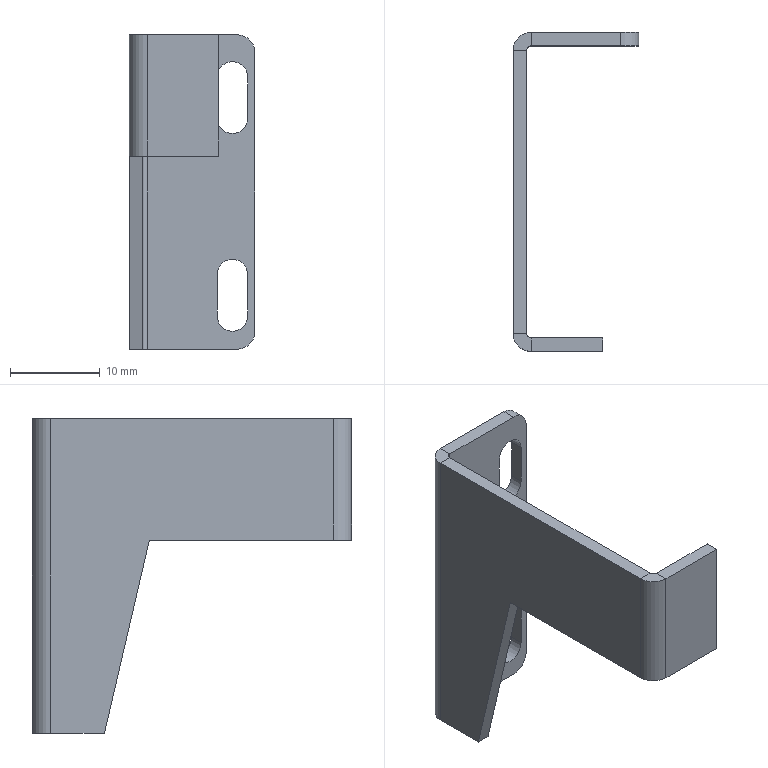Part | NX | features BREP 1 | 1 solid | 36 faces | box 14 x 35.5 x 35 mm | volume 1770 mm3 | plane 24 | cylinder 12 | commonest cylinder face diameters 3.4 x6 4 x4 1 x2
STEP:
#1=CARTESIAN_POINT('',(12.,0.,17.5));
#2=VERTEX_POINT('',#1);
#3=CARTESIAN_POINT('',(14.,0.,15.5));
#4=VERTEX_POINT('',#3);
#5=CARTESIAN_POINT('',(12.,0.,15.5));
#6=DIRECTION('',(0.,1.,0.));
#7=DIRECTION('',(0.,0.,1.));
#8=AXIS2_PLACEMENT_3D('',#5,#6,#7);
#9=CIRCLE('',#8,2.);
#10=EDGE_CURVE('',#2,#4,#9,.T.);
#11=ORIENTED_EDGE('',*,*,#10,.F.);
#12=CARTESIAN_POINT('',(12.,-1.5,17.5));
#13=VERTEX_POINT('',#12);
#14=CARTESIAN_POINT('',(12.,-2.,17.5));
#15=DIRECTION('',(0.,1.,0.));
#16=VECTOR('',#15,1000.);
#17=LINE('',#14,#16);
#18=EDGE_CURVE('',#13,#2,#17,.T.);
#19=ORIENTED_EDGE('',*,*,#18,.F.);
#20=CARTESIAN_POINT('',(14.,-1.5,15.5));
#21=VERTEX_POINT('',#20);
#22=CARTESIAN_POINT('',(12.,-1.5,15.5));
#23=DIRECTION('',(0.,-1.,0.));
#24=DIRECTION('',(0.,0.,1.));
#25=AXIS2_PLACEMENT_3D('',#22,#23,#24);
#26=CIRCLE('',#25,2.);
#27=EDGE_CURVE('',#21,#13,#26,.T.);
#28=ORIENTED_EDGE('',*,*,#27,.F.);
#29=CARTESIAN_POINT('',(14.,0.,15.5));
#30=DIRECTION('',(0.,-1.,0.));
#31=VECTOR('',#30,1000.);
#32=LINE('',#29,#31);
#33=EDGE_CURVE('',#4,#21,#32,.T.);
#34=ORIENTED_EDGE('',*,*,#33,.F.);
#35=EDGE_LOOP('',(#11,#19,#28,#34));
#36=FACE_BOUND('',#35,.T.);
#37=CARTESIAN_POINT('',(12.,0.,15.5));
#38=DIRECTION('',(0.,-1.,0.));
#39=DIRECTION('',(0.,0.,-1.));
#40=AXIS2_PLACEMENT_3D('',#37,#38,#39);
#41=CYLINDRICAL_SURFACE('',#40,2.);
#42=ADVANCED_FACE('',(#36),#41,.T.);
#43=CARTESIAN_POINT('',(14.,0.,-15.5));
#44=VERTEX_POINT('',#43);
#45=CARTESIAN_POINT('',(12.,0.,-17.5));
#46=VERTEX_POINT('',#45);
#47=CARTESIAN_POINT('',(12.,0.,-15.5));
#48=DIRECTION('',(0.,1.,0.));
#49=DIRECTION('',(0.,0.,1.));
#50=AXIS2_PLACEMENT_3D('',#47,#48,#49);
#51=CIRCLE('',#50,2.);
#52=EDGE_CURVE('',#44,#46,#51,.T.);
#53=ORIENTED_EDGE('',*,*,#52,.F.);
#54=CARTESIAN_POINT('',(14.,-1.5,-15.5));
#55=VERTEX_POINT('',#54);
#56=CARTESIAN_POINT('',(14.,0.,-15.5));
#57=DIRECTION('',(0.,1.,0.));
#58=VECTOR('',#57,1000.);
#59=LINE('',#56,#58);
#60=EDGE_CURVE('',#55,#44,#59,.T.);
#61=ORIENTED_EDGE('',*,*,#60,.F.);
#62=CARTESIAN_POINT('',(12.,-1.5,-17.5));
#63=VERTEX_POINT('',#62);
#64=CARTESIAN_POINT('',(12.,-1.5,-15.5));
#65=DIRECTION('',(0.,-1.,0.));
#66=DIRECTION('',(0.,0.,1.));
#67=AXIS2_PLACEMENT_3D('',#64,#65,#66);
#68=CIRCLE('',#67,2.);
#69=EDGE_CURVE('',#63,#55,#68,.T.);
#70=ORIENTED_EDGE('',*,*,#69,.F.);
#71=CARTESIAN_POINT('',(12.,-1.5,-17.5));
#72=DIRECTION('',(0.,-1.,0.));
#73=VECTOR('',#72,1000.);
#74=LINE('',#71,#73);
#75=EDGE_CURVE('',#46,#63,#74,.T.);
#76=ORIENTED_EDGE('',*,*,#75,.F.);
#77=EDGE_LOOP('',(#53,#61,#70,#76));
#78=FACE_BOUND('',#77,.T.);
#79=CARTESIAN_POINT('',(12.,-2.,-15.5));
#80=DIRECTION('',(0.,1.,0.));
#81=DIRECTION('',(0.,0.,1.));
#82=AXIS2_PLACEMENT_3D('',#79,#80,#81);
#83=CYLINDRICAL_SURFACE('',#82,2.);
#84=ADVANCED_FACE('',(#78),#83,.T.);
#85=CARTESIAN_POINT('',(13.2,0.,-9.2));
#86=VERTEX_POINT('',#85);
#87=CARTESIAN_POINT('',(13.2,-1.5,-9.2));
#88=VERTEX_POINT('',#87);
#89=CARTESIAN_POINT('',(13.2,-1.501,-9.2));
#90=DIRECTION('',(0.,-1.,0.));
#91=VECTOR('',#90,1000.);
#92=LINE('',#89,#91);
#93=EDGE_CURVE('',#86,#88,#92,.T.);
#94=ORIENTED_EDGE('',*,*,#93,.F.);
#95=CARTESIAN_POINT('',(13.2,0.,-13.8));
#96=VERTEX_POINT('',#95);
#97=CARTESIAN_POINT('',(13.2,0.,-9.2));
#98=DIRECTION('',(0.,0.,-1.));
#99=VECTOR('',#98,1000.);
#100=LINE('',#97,#99);
#101=EDGE_CURVE('',#86,#96,#100,.T.);
#102=ORIENTED_EDGE('',*,*,#101,.T.);
#103=CARTESIAN_POINT('',(13.2,-1.5,-13.8));
#104=VERTEX_POINT('',#103);
#105=CARTESIAN_POINT('',(13.2,-1.501,-13.8));
#106=DIRECTION('',(0.,-1.,0.));
#107=VECTOR('',#106,1000.);
#108=LINE('',#105,#107);
#109=EDGE_CURVE('',#96,#104,#108,.T.);
#110=ORIENTED_EDGE('',*,*,#109,.T.);
#111=CARTESIAN_POINT('',(13.2,-1.5,17.5));
#112=DIRECTION('',(0.,0.,-1.));
#113=VECTOR('',#112,1000.);
#114=LINE('',#111,#113);
#115=EDGE_CURVE('',#88,#104,#114,.T.);
#116=ORIENTED_EDGE('',*,*,#115,.F.);
#117=EDGE_LOOP('',(#94,#102,#110,#116));
#118=FACE_BOUND('',#117,.T.);
#119=CARTESIAN_POINT('',(13.2,-1.501,-9.2));
#120=DIRECTION('',(1.,0.,0.));
#121=DIRECTION('',(0.,1.,0.));
#122=AXIS2_PLACEMENT_3D('',#119,#120,#121);
#123=PLANE('',#122);
#124=ADVANCED_FACE('',(#118),#123,.F.);
#125=CARTESIAN_POINT('',(9.8,-1.5,-13.8));
#126=VERTEX_POINT('',#125);
#127=CARTESIAN_POINT('',(9.8,0.,-13.8));
#128=VERTEX_POINT('',#127);
#129=CARTESIAN_POINT('',(9.8,0.,-13.8));
#130=DIRECTION('',(0.,1.,0.));
#131=VECTOR('',#130,1000.);
#132=LINE('',#129,#131);
#133=EDGE_CURVE('',#126,#128,#132,.T.);
#134=ORIENTED_EDGE('',*,*,#133,.T.);
#135=CARTESIAN_POINT('',(9.8,0.,-9.2));
#136=VERTEX_POINT('',#135);
#137=CARTESIAN_POINT('',(9.8,0.,-9.2));
#138=DIRECTION('',(0.,0.,-1.));
#139=VECTOR('',#138,1000.);
#140=LINE('',#137,#139);
#141=EDGE_CURVE('',#136,#128,#140,.T.);
#142=ORIENTED_EDGE('',*,*,#141,.F.);
#143=CARTESIAN_POINT('',(9.8,-1.5,-9.2));
#144=VERTEX_POINT('',#143);
#145=CARTESIAN_POINT('',(9.8,0.,-9.2));
#146=DIRECTION('',(0.,-1.,0.));
#147=VECTOR('',#146,1000.);
#148=LINE('',#145,#147);
#149=EDGE_CURVE('',#136,#144,#148,.T.);
#150=ORIENTED_EDGE('',*,*,#149,.T.);
#151=CARTESIAN_POINT('',(9.8,-1.5,17.5));
#152=DIRECTION('',(0.,0.,1.));
#153=VECTOR('',#152,1000.);
#154=LINE('',#151,#153);
#155=EDGE_CURVE('',#126,#144,#154,.T.);
#156=ORIENTED_EDGE('',*,*,#155,.F.);
#157=EDGE_LOOP('',(#134,#142,#150,#156));
#158=FACE_BOUND('',#157,.T.);
#159=CARTESIAN_POINT('',(9.8,0.,-9.2));
#160=DIRECTION('',(-1.,0.,0.));
#161=DIRECTION('',(0.,0.,1.));
#162=AXIS2_PLACEMENT_3D('',#159,#160,#161);
#163=PLANE('',#162);
#164=ADVANCED_FACE('',(#158),#163,.F.);
#165=CARTESIAN_POINT('',(11.5,-1.5,-7.5));
#166=VERTEX_POINT('',#165);
#167=CARTESIAN_POINT('',(11.5,0.,-7.5));
#168=VERTEX_POINT('',#167);
#169=CARTESIAN_POINT('',(11.5,0.,-7.5));
#170=DIRECTION('',(0.,1.,0.));
#171=VECTOR('',#170,1000.);
#172=LINE('',#169,#171);
#173=EDGE_CURVE('',#166,#168,#172,.T.);
#174=ORIENTED_EDGE('',*,*,#173,.F.);
#175=CARTESIAN_POINT('',(11.5,-1.5,-9.2));
#176=DIRECTION('',(0.,1.,0.));
#177=DIRECTION('',(0.,0.,1.));
#178=AXIS2_PLACEMENT_3D('',#175,#176,#177);
#179=CIRCLE('',#178,1.7);
#180=EDGE_CURVE('',#144,#166,#179,.T.);
#181=ORIENTED_EDGE('',*,*,#180,.F.);
#182=ORIENTED_EDGE('',*,*,#149,.F.);
#183=CARTESIAN_POINT('',(11.5,0.,-9.2));
#184=DIRECTION('',(0.,1.,0.));
#185=DIRECTION('',(0.,0.,1.));
#186=AXIS2_PLACEMENT_3D('',#183,#184,#185);
#187=CIRCLE('',#186,1.7);
#188=EDGE_CURVE('',#136,#168,#187,.T.);
#189=ORIENTED_EDGE('',*,*,#188,.T.);
#190=EDGE_LOOP('',(#174,#181,#182,#189));
#191=FACE_BOUND('',#190,.T.);
#192=CARTESIAN_POINT('',(11.5,0.,-9.2));
#193=DIRECTION('',(0.,1.,0.));
#194=DIRECTION('',(0.,0.,1.));
#195=AXIS2_PLACEMENT_3D('',#192,#193,#194);
#196=CYLINDRICAL_SURFACE('',#195,1.7);
#197=ADVANCED_FACE('',(#191),#196,.F.);
#198=ORIENTED_EDGE('',*,*,#109,.F.);
#199=CARTESIAN_POINT('',(11.5,0.,-13.8));
#200=DIRECTION('',(0.,1.,0.));
#201=DIRECTION('',(0.,0.,1.));
#202=AXIS2_PLACEMENT_3D('',#199,#200,#201);
#203=CIRCLE('',#202,1.7);
#204=EDGE_CURVE('',#96,#128,#203,.T.);
#205=ORIENTED_EDGE('',*,*,#204,.T.);
#206=ORIENTED_EDGE('',*,*,#133,.F.);
#207=CARTESIAN_POINT('',(11.5,-1.5,-13.8));
#208=DIRECTION('',(0.,1.,0.));
#209=DIRECTION('',(0.,0.,1.));
#210=AXIS2_PLACEMENT_3D('',#207,#208,#209);
#211=CIRCLE('',#210,1.7);
#212=EDGE_CURVE('',#104,#126,#211,.T.);
#213=ORIENTED_EDGE('',*,*,#212,.F.);
#214=EDGE_LOOP('',(#198,#205,#206,#213));
#215=FACE_BOUND('',#214,.T.);
#216=CARTESIAN_POINT('',(11.5,0.,-13.8));
#217=DIRECTION('',(0.,1.,0.));
#218=DIRECTION('',(0.,0.,1.));
#219=AXIS2_PLACEMENT_3D('',#216,#217,#218);
#220=CYLINDRICAL_SURFACE('',#219,1.7);
#221=ADVANCED_FACE('',(#215),#220,.F.);
#222=CARTESIAN_POINT('',(13.2,0.,12.8));
#223=VERTEX_POINT('',#222);
#224=CARTESIAN_POINT('',(13.2,-1.5,12.8));
#225=VERTEX_POINT('',#224);
#226=CARTESIAN_POINT('',(13.2,-1.501,12.8));
#227=DIRECTION('',(0.,-1.,0.));
#228=VECTOR('',#227,1000.);
#229=LINE('',#226,#228);
#230=EDGE_CURVE('',#223,#225,#229,.T.);
#231=ORIENTED_EDGE('',*,*,#230,.F.);
#232=CARTESIAN_POINT('',(13.2,0.,8.2));
#233=VERTEX_POINT('',#232);
#234=CARTESIAN_POINT('',(13.2,0.,12.8));
#235=DIRECTION('',(0.,0.,-1.));
#236=VECTOR('',#235,1000.);
#237=LINE('',#234,#236);
#238=EDGE_CURVE('',#223,#233,#237,.T.);
#239=ORIENTED_EDGE('',*,*,#238,.T.);
#240=CARTESIAN_POINT('',(13.2,-1.5,8.2));
#241=VERTEX_POINT('',#240);
#242=CARTESIAN_POINT('',(13.2,-1.501,8.2));
#243=DIRECTION('',(0.,-1.,0.));
#244=VECTOR('',#243,1000.);
#245=LINE('',#242,#244);
#246=EDGE_CURVE('',#233,#241,#245,.T.);
#247=ORIENTED_EDGE('',*,*,#246,.T.);
#248=CARTESIAN_POINT('',(13.2,-1.5,17.5));
#249=DIRECTION('',(0.,0.,-1.));
#250=VECTOR('',#249,1000.);
#251=LINE('',#248,#250);
#252=EDGE_CURVE('',#225,#241,#251,.T.);
#253=ORIENTED_EDGE('',*,*,#252,.F.);
#254=EDGE_LOOP('',(#231,#239,#247,#253));
#255=FACE_BOUND('',#254,.T.);
#256=CARTESIAN_POINT('',(13.2,-1.501,12.8));
#257=DIRECTION('',(1.,0.,0.));
#258=DIRECTION('',(0.,1.,0.));
#259=AXIS2_PLACEMENT_3D('',#256,#257,#258);
#260=PLANE('',#259);
#261=ADVANCED_FACE('',(#255),#260,.F.);
#262=CARTESIAN_POINT('',(9.8,-1.5,8.2));
#263=VERTEX_POINT('',#262);
#264=CARTESIAN_POINT('',(9.8,0.,8.2));
#265=VERTEX_POINT('',#264);
#266=CARTESIAN_POINT('',(9.8,0.,8.2));
#267=DIRECTION('',(0.,1.,0.));
#268=VECTOR('',#267,1000.);
#269=LINE('',#266,#268);
#270=EDGE_CURVE('',#263,#265,#269,.T.);
#271=ORIENTED_EDGE('',*,*,#270,.T.);
#272=CARTESIAN_POINT('',(9.8,0.,12.8));
#273=VERTEX_POINT('',#272);
#274=CARTESIAN_POINT('',(9.8,0.,12.8));
#275=DIRECTION('',(0.,0.,-1.));
#276=VECTOR('',#275,1000.);
#277=LINE('',#274,#276);
#278=EDGE_CURVE('',#273,#265,#277,.T.);
#279=ORIENTED_EDGE('',*,*,#278,.F.);
#280=CARTESIAN_POINT('',(9.8,-1.5,12.8));
#281=VERTEX_POINT('',#280);
#282=CARTESIAN_POINT('',(9.8,0.,12.8));
#283=DIRECTION('',(0.,-1.,0.));
#284=VECTOR('',#283,1000.);
#285=LINE('',#282,#284);
#286=EDGE_CURVE('',#273,#281,#285,.T.);
#287=ORIENTED_EDGE('',*,*,#286,.T.);
#288=CARTESIAN_POINT('',(9.8,-1.5,17.5));
#289=DIRECTION('',(0.,0.,1.));
#290=VECTOR('',#289,1000.);
#291=LINE('',#288,#290);
#292=EDGE_CURVE('',#263,#281,#291,.T.);
#293=ORIENTED_EDGE('',*,*,#292,.F.);
#294=EDGE_LOOP('',(#271,#279,#287,#293));
#295=FACE_BOUND('',#294,.T.);
#296=CARTESIAN_POINT('',(9.8,0.,12.8));
#297=DIRECTION('',(-1.,0.,0.));
#298=DIRECTION('',(0.,0.,1.));
#299=AXIS2_PLACEMENT_3D('',#296,#297,#298);
#300=PLANE('',#299);
#301=ADVANCED_FACE('',(#295),#300,.F.);
#302=CARTESIAN_POINT('',(11.5,-1.5,14.5));
#303=VERTEX_POINT('',#302);
#304=CARTESIAN_POINT('',(11.5,0.,14.5));
#305=VERTEX_POINT('',#304);
#306=CARTESIAN_POINT('',(11.5,0.,14.5));
#307=DIRECTION('',(0.,1.,0.));
#308=VECTOR('',#307,1000.);
#309=LINE('',#306,#308);
#310=EDGE_CURVE('',#303,#305,#309,.T.);
#311=ORIENTED_EDGE('',*,*,#310,.F.);
#312=CARTESIAN_POINT('',(11.5,-1.5,12.8));
#313=DIRECTION('',(0.,1.,0.));
#314=DIRECTION('',(0.,0.,1.));
#315=AXIS2_PLACEMENT_3D('',#312,#313,#314);
#316=CIRCLE('',#315,1.7);
#317=EDGE_CURVE('',#281,#303,#316,.T.);
#318=ORIENTED_EDGE('',*,*,#317,.F.);
#319=ORIENTED_EDGE('',*,*,#286,.F.);
#320=CARTESIAN_POINT('',(11.5,0.,12.8));
#321=DIRECTION('',(0.,1.,0.));
#322=DIRECTION('',(0.,0.,1.));
#323=AXIS2_PLACEMENT_3D('',#320,#321,#322);
#324=CIRCLE('',#323,1.7);
#325=EDGE_CURVE('',#273,#305,#324,.T.);
#326=ORIENTED_EDGE('',*,*,#325,.T.);
#327=EDGE_LOOP('',(#311,#318,#319,#326));
#328=FACE_BOUND('',#327,.T.);
#329=CARTESIAN_POINT('',(11.5,0.,12.8));
#330=DIRECTION('',(0.,1.,0.));
#331=DIRECTION('',(0.,0.,1.));
#332=AXIS2_PLACEMENT_3D('',#329,#330,#331);
#333=CYLINDRICAL_SURFACE('',#332,1.7);
#334=ADVANCED_FACE('',(#328),#333,.F.);
#335=ORIENTED_EDGE('',*,*,#246,.F.);
#336=CARTESIAN_POINT('',(11.5,0.,8.2));
#337=DIRECTION('',(0.,1.,0.));
#338=DIRECTION('',(0.,0.,1.));
#339=AXIS2_PLACEMENT_3D('',#336,#337,#338);
#340=CIRCLE('',#339,1.7);
#341=EDGE_CURVE('',#233,#265,#340,.T.);
#342=ORIENTED_EDGE('',*,*,#341,.T.);
#343=ORIENTED_EDGE('',*,*,#270,.F.);
#344=CARTESIAN_POINT('',(11.5,-1.5,8.2));
#345=DIRECTION('',(0.,1.,0.));
#346=DIRECTION('',(0.,0.,1.));
#347=AXIS2_PLACEMENT_3D('',#344,#345,#346);
#348=CIRCLE('',#347,1.7);
#349=EDGE_CURVE('',#241,#263,#348,.T.);
#350=ORIENTED_EDGE('',*,*,#349,.F.);
#351=EDGE_LOOP('',(#335,#342,#343,#350));
#352=FACE_BOUND('',#351,.T.);
#353=CARTESIAN_POINT('',(11.5,0.,8.2));
#354=DIRECTION('',(0.,1.,0.));
#355=DIRECTION('',(0.,0.,1.));
#356=AXIS2_PLACEMENT_3D('',#353,#354,#355);
#357=CYLINDRICAL_SURFACE('',#356,1.7);
#358=ADVANCED_FACE('',(#352),#357,.F.);
#359=CARTESIAN_POINT('',(2.,-35.5,4.));
#360=VERTEX_POINT('',#359);
#361=CARTESIAN_POINT('',(2.,-34.,4.));
#362=VERTEX_POINT('',#361);
#363=CARTESIAN_POINT('',(2.,-35.5,4.));
#364=DIRECTION('',(0.,1.,0.));
#365=VECTOR('',#364,1000.);
#366=LINE('',#363,#365);
#367=EDGE_CURVE('',#360,#362,#366,.T.);
#368=ORIENTED_EDGE('',*,*,#367,.F.);
#369=CARTESIAN_POINT('',(0.,-33.5,4.));
#370=VERTEX_POINT('',#369);
#371=CARTESIAN_POINT('',(2.,-33.5,4.));
#372=DIRECTION('',(0.,0.,1.));
#373=DIRECTION('',(0.,1.,0.));
#374=AXIS2_PLACEMENT_3D('',#371,#372,#373);
#375=CIRCLE('',#374,2.);
#376=EDGE_CURVE('',#370,#360,#375,.T.);
#377=ORIENTED_EDGE('',*,*,#376,.F.);
#378=CARTESIAN_POINT('',(1.5,-33.5,4.));
#379=VERTEX_POINT('',#378);
#380=CARTESIAN_POINT('',(1.5,-33.5,4.));
#381=DIRECTION('',(-1.,0.,0.));
#382=VECTOR('',#381,1000.);
#383=LINE('',#380,#382);
#384=EDGE_CURVE('',#379,#370,#383,.T.);
#385=ORIENTED_EDGE('',*,*,#384,.F.);
#386=CARTESIAN_POINT('',(2.,-33.5,4.));
#387=DIRECTION('',(0.,0.,1.));
#388=DIRECTION('',(-1.,0.,0.));
#389=AXIS2_PLACEMENT_3D('',#386,#387,#388);
#390=CIRCLE('',#389,0.5);
#391=EDGE_CURVE('',#379,#362,#390,.T.);
#392=ORIENTED_EDGE('',*,*,#391,.T.);
#393=EDGE_LOOP('',(#368,#377,#385,#392));
#394=FACE_BOUND('',#393,.T.);
#395=CARTESIAN_POINT('',(2.,-33.5,4.));
#396=DIRECTION('',(0.,0.,1.));
#397=DIRECTION('',(0.,-1.,0.));
#398=AXIS2_PLACEMENT_3D('',#395,#396,#397);
#399=PLANE('',#398);
#400=ADVANCED_FACE('',(#394),#399,.F.);
#401=CARTESIAN_POINT('',(10.,-35.5,4.));
#402=VERTEX_POINT('',#401);
#403=CARTESIAN_POINT('',(10.,-34.,4.));
#404=VERTEX_POINT('',#403);
#405=CARTESIAN_POINT('',(10.,-35.5,4.));
#406=DIRECTION('',(0.,1.,0.));
#407=VECTOR('',#406,1000.);
#408=LINE('',#405,#407);
#409=EDGE_CURVE('',#402,#404,#408,.T.);
#410=ORIENTED_EDGE('',*,*,#409,.F.);
#411=CARTESIAN_POINT('',(14.,-35.5,4.));
#412=DIRECTION('',(-1.,0.,0.));
#413=VECTOR('',#412,1000.);
#414=LINE('',#411,#413);
#415=EDGE_CURVE('',#402,#360,#414,.T.);
#416=ORIENTED_EDGE('',*,*,#415,.T.);
#417=ORIENTED_EDGE('',*,*,#367,.T.);
#418=CARTESIAN_POINT('',(0.,-34.,4.));
#419=DIRECTION('',(-1.,0.,0.));
#420=VECTOR('',#419,1000.);
#421=LINE('',#418,#420);
#422=EDGE_CURVE('',#404,#362,#421,.T.);
#423=ORIENTED_EDGE('',*,*,#422,.F.);
#424=EDGE_LOOP('',(#410,#416,#417,#423));
#425=FACE_BOUND('',#424,.T.);
#426=CARTESIAN_POINT('',(14.,-35.5,4.));
#427=DIRECTION('',(0.,0.,1.));
#428=DIRECTION('',(-1.,0.,0.));
#429=AXIS2_PLACEMENT_3D('',#426,#427,#428);
#430=PLANE('',#429);
#431=ADVANCED_FACE('',(#425),#430,.F.);
#432=CARTESIAN_POINT('',(1.5,-8.,-17.5));
#433=VERTEX_POINT('',#432);
#434=CARTESIAN_POINT('',(1.5,-13.,4.));
#435=VERTEX_POINT('',#434);
#436=CARTESIAN_POINT('',(1.5,-15.311,13.939));
#437=DIRECTION('',(0.,-0.2265,0.974));
#438=VECTOR('',#437,1000.);
#439=LINE('',#436,#438);
#440=EDGE_CURVE('',#433,#435,#439,.T.);
#441=ORIENTED_EDGE('',*,*,#440,.T.);
#442=CARTESIAN_POINT('',(0.,-13.,4.));
#443=VERTEX_POINT('',#442);
#444=CARTESIAN_POINT('',(1.5,-13.,4.));
#445=DIRECTION('',(-1.,0.,0.));
#446=VECTOR('',#445,1000.);
#447=LINE('',#444,#446);
#448=EDGE_CURVE('',#435,#443,#447,.T.);
#449=ORIENTED_EDGE('',*,*,#448,.T.);
#450=CARTESIAN_POINT('',(0.,-8.,-17.5));
#451=VERTEX_POINT('',#450);
#452=CARTESIAN_POINT('',(0.,-15.311,13.939));
#453=DIRECTION('',(0.,-0.2265,0.974));
#454=VECTOR('',#453,1000.);
#455=LINE('',#452,#454);
#456=EDGE_CURVE('',#451,#443,#455,.T.);
#457=ORIENTED_EDGE('',*,*,#456,.F.);
#458=CARTESIAN_POINT('',(1.5,-8.,-17.5));
#459=DIRECTION('',(-1.,0.,0.));
#460=VECTOR('',#459,1000.);
#461=LINE('',#458,#460);
#462=EDGE_CURVE('',#433,#451,#461,.T.);
#463=ORIENTED_EDGE('',*,*,#462,.F.);
#464=EDGE_LOOP('',(#441,#449,#457,#463));
#465=FACE_BOUND('',#464,.T.);
#466=CARTESIAN_POINT('',(1.5,-15.311,13.939));
#467=DIRECTION('',(0.,-0.974,-0.2265));
#468=DIRECTION('',(0.,-0.2265,0.974));
#469=AXIS2_PLACEMENT_3D('',#466,#467,#468);
#470=PLANE('',#469);
#471=ADVANCED_FACE('',(#465),#470,.T.);
#472=ORIENTED_EDGE('',*,*,#448,.F.);
#473=CARTESIAN_POINT('',(1.5,0.,4.));
#474=DIRECTION('',(0.,-1.,0.));
#475=VECTOR('',#474,1000.);
#476=LINE('',#473,#475);
#477=EDGE_CURVE('',#435,#379,#476,.T.);
#478=ORIENTED_EDGE('',*,*,#477,.T.);
#479=ORIENTED_EDGE('',*,*,#384,.T.);
#480=CARTESIAN_POINT('',(0.,0.,4.));
#481=DIRECTION('',(0.,-1.,0.));
#482=VECTOR('',#481,1000.);
#483=LINE('',#480,#482);
#484=EDGE_CURVE('',#443,#370,#483,.T.);
#485=ORIENTED_EDGE('',*,*,#484,.F.);
#486=EDGE_LOOP('',(#472,#478,#479,#485));
#487=FACE_BOUND('',#486,.T.);
#488=CARTESIAN_POINT('',(1.5,0.,4.));
#489=DIRECTION('',(0.,0.,-1.));
#490=DIRECTION('',(0.,-1.,0.));
#491=AXIS2_PLACEMENT_3D('',#488,#489,#490);
#492=PLANE('',#491);
#493=ADVANCED_FACE('',(#487),#492,.T.);
#494=CARTESIAN_POINT('',(2.,0.,-17.5));
#495=VERTEX_POINT('',#494);
#496=CARTESIAN_POINT('',(0.,0.,-17.5));
#497=DIRECTION('',(1.,0.,0.));
#498=VECTOR('',#497,1000.);
#499=LINE('',#496,#498);
#500=EDGE_CURVE('',#495,#46,#499,.T.);
#501=ORIENTED_EDGE('',*,*,#500,.T.);
#502=ORIENTED_EDGE('',*,*,#75,.T.);
#503=CARTESIAN_POINT('',(2.,-1.5,-17.5));
#504=VERTEX_POINT('',#503);
#505=CARTESIAN_POINT('',(0.,-1.5,-17.5));
#506=DIRECTION('',(1.,0.,0.));
#507=VECTOR('',#506,1000.);
#508=LINE('',#505,#507);
#509=EDGE_CURVE('',#504,#63,#508,.T.);
#510=ORIENTED_EDGE('',*,*,#509,.F.);
#511=CARTESIAN_POINT('',(2.,-1.5,-17.5));
#512=DIRECTION('',(0.,1.,0.));
#513=VECTOR('',#512,1000.);
#514=LINE('',#511,#513);
#515=EDGE_CURVE('',#504,#495,#514,.T.);
#516=ORIENTED_EDGE('',*,*,#515,.T.);
#517=EDGE_LOOP('',(#501,#502,#510,#516));
#518=FACE_BOUND('',#517,.T.);
#519=CARTESIAN_POINT('',(2.,-2.,-17.5));
#520=DIRECTION('',(0.,0.,1.));
#521=DIRECTION('',(1.,0.,0.));
#522=AXIS2_PLACEMENT_3D('',#519,#520,#521);
#523=PLANE('',#522);
#524=ADVANCED_FACE('',(#518),#523,.F.);
#525=CARTESIAN_POINT('',(10.,-34.,17.5));
#526=VERTEX_POINT('',#525);
#527=CARTESIAN_POINT('',(2.,-34.,17.5));
#528=VERTEX_POINT('',#527);
#529=CARTESIAN_POINT('',(0.,-34.,17.5));
#530=DIRECTION('',(-1.,0.,0.));
#531=VECTOR('',#530,1000.);
#532=LINE('',#529,#531);
#533=EDGE_CURVE('',#526,#528,#532,.T.);
#534=ORIENTED_EDGE('',*,*,#533,.T.);
#535=CARTESIAN_POINT('',(2.,-35.5,17.5));
#536=VERTEX_POINT('',#535);
#537=CARTESIAN_POINT('',(2.,-34.,17.5));
#538=DIRECTION('',(0.,-1.,0.));
#539=VECTOR('',#538,1000.);
#540=LINE('',#537,#539);
#541=EDGE_CURVE('',#528,#536,#540,.T.);
#542=ORIENTED_EDGE('',*,*,#541,.T.);
#543=CARTESIAN_POINT('',(10.,-35.5,17.5));
#544=VERTEX_POINT('',#543);
#545=CARTESIAN_POINT('',(0.,-35.5,17.5));
#546=DIRECTION('',(-1.,0.,0.));
#547=VECTOR('',#546,1000.);
#548=LINE('',#545,#547);
#549=EDGE_CURVE('',#544,#536,#548,.T.);
#550=ORIENTED_EDGE('',*,*,#549,.F.);
#551=CARTESIAN_POINT('',(10.,-34.,17.5));
#552=DIRECTION('',(0.,-1.,0.));
#553=VECTOR('',#552,1000.);
#554=LINE('',#551,#553);
#555=EDGE_CURVE('',#526,#544,#554,.T.);
#556=ORIENTED_EDGE('',*,*,#555,.F.);
#557=EDGE_LOOP('',(#534,#542,#550,#556));
#558=FACE_BOUND('',#557,.T.);
#559=CARTESIAN_POINT('',(2.,-2.,17.5));
#560=DIRECTION('',(0.,0.,1.));
#561=DIRECTION('',(1.,0.,0.));
#562=AXIS2_PLACEMENT_3D('',#559,#560,#561);
#563=PLANE('',#562);
#564=ADVANCED_FACE('',(#558),#563,.T.);
#565=CARTESIAN_POINT('',(1.5,-2.,-17.5));
#566=VERTEX_POINT('',#565);
#567=CARTESIAN_POINT('',(2.,-2.,-17.5));
#568=DIRECTION('',(0.,0.,-1.));
#569=DIRECTION('',(1.,0.,0.));
#570=AXIS2_PLACEMENT_3D('',#567,#568,#569);
#571=CIRCLE('',#570,0.5);
#572=EDGE_CURVE('',#566,#504,#571,.T.);
#573=ORIENTED_EDGE('',*,*,#572,.T.);
#574=CARTESIAN_POINT('',(2.,-1.5,17.5));
#575=VERTEX_POINT('',#574);
#576=CARTESIAN_POINT('',(2.,-1.5,17.5));
#577=DIRECTION('',(0.,0.,-1.));
#578=VECTOR('',#577,1000.);
#579=LINE('',#576,#578);
#580=EDGE_CURVE('',#575,#504,#579,.T.);
#581=ORIENTED_EDGE('',*,*,#580,.F.);
#582=CARTESIAN_POINT('',(1.5,-2.,17.5));
#583=VERTEX_POINT('',#582);
#584=CARTESIAN_POINT('',(2.,-2.,17.5));
#585=DIRECTION('',(0.,0.,-1.));
#586=DIRECTION('',(1.,0.,0.));
#587=AXIS2_PLACEMENT_3D('',#584,#585,#586);
#588=CIRCLE('',#587,0.5);
#589=EDGE_CURVE('',#583,#575,#588,.T.);
#590=ORIENTED_EDGE('',*,*,#589,.F.);
#591=CARTESIAN_POINT('',(1.5,-2.,17.5));
#592=DIRECTION('',(0.,0.,-1.));
#593=VECTOR('',#592,1000.);
#594=LINE('',#591,#593);
#595=EDGE_CURVE('',#583,#566,#594,.T.);
#596=ORIENTED_EDGE('',*,*,#595,.T.);
#597=EDGE_LOOP('',(#573,#581,#590,#596));
#598=FACE_BOUND('',#597,.T.);
#599=CARTESIAN_POINT('',(2.,-2.,17.5));
#600=DIRECTION('',(0.,0.,-1.));
#601=DIRECTION('',(-1.,0.,0.));
#602=AXIS2_PLACEMENT_3D('',#599,#600,#601);
#603=CYLINDRICAL_SURFACE('',#602,0.5);
#604=ADVANCED_FACE('',(#598),#603,.F.);
#605=CARTESIAN_POINT('',(0.,-2.,-17.5));
#606=VERTEX_POINT('',#605);
#607=CARTESIAN_POINT('',(2.,-2.,-17.5));
#608=DIRECTION('',(0.,0.,-1.));
#609=DIRECTION('',(1.,0.,0.));
#610=AXIS2_PLACEMENT_3D('',#607,#608,#609);
#611=CIRCLE('',#610,2.);
#612=EDGE_CURVE('',#606,#495,#611,.T.);
#613=ORIENTED_EDGE('',*,*,#612,.F.);
#614=CARTESIAN_POINT('',(0.,-2.,17.5));
#615=VERTEX_POINT('',#614);
#616=CARTESIAN_POINT('',(0.,-2.,17.5));
#617=DIRECTION('',(0.,0.,-1.));
#618=VECTOR('',#617,1000.);
#619=LINE('',#616,#618);
#620=EDGE_CURVE('',#615,#606,#619,.T.);
#621=ORIENTED_EDGE('',*,*,#620,.F.);
#622=CARTESIAN_POINT('',(2.,0.,17.5));
#623=VERTEX_POINT('',#622);
#624=CARTESIAN_POINT('',(2.,-2.,17.5));
#625=DIRECTION('',(0.,0.,-1.));
#626=DIRECTION('',(1.,0.,0.));
#627=AXIS2_PLACEMENT_3D('',#624,#625,#626);
#628=CIRCLE('',#627,2.);
#629=EDGE_CURVE('',#615,#623,#628,.T.);
#630=ORIENTED_EDGE('',*,*,#629,.T.);
#631=CARTESIAN_POINT('',(2.,0.,17.5));
#632=DIRECTION('',(0.,0.,-1.));
#633=VECTOR('',#632,1000.);
#634=LINE('',#631,#633);
#635=EDGE_CURVE('',#623,#495,#634,.T.);
#636=ORIENTED_EDGE('',*,*,#635,.T.);
#637=EDGE_LOOP('',(#613,#621,#630,#636));
#638=FACE_BOUND('',#637,.T.);
#639=CARTESIAN_POINT('',(2.,-2.,17.5));
#640=DIRECTION('',(0.,0.,-1.));
#641=DIRECTION('',(-1.,0.,0.));
#642=AXIS2_PLACEMENT_3D('',#639,#640,#641);
#643=CYLINDRICAL_SURFACE('',#642,2.);
#644=ADVANCED_FACE('',(#638),#643,.T.);
#645=CARTESIAN_POINT('',(14.,0.,17.5));
#646=DIRECTION('',(0.,0.,-1.));
#647=VECTOR('',#646,1000.);
#648=LINE('',#645,#647);
#649=EDGE_CURVE('',#4,#44,#648,.T.);
#650=ORIENTED_EDGE('',*,*,#649,.T.);
#651=ORIENTED_EDGE('',*,*,#52,.T.);
#652=ORIENTED_EDGE('',*,*,#500,.F.);
#653=ORIENTED_EDGE('',*,*,#635,.F.);
#654=CARTESIAN_POINT('',(0.,0.,17.5));
#655=DIRECTION('',(1.,0.,0.));
#656=VECTOR('',#655,1000.);
#657=LINE('',#654,#656);
#658=EDGE_CURVE('',#623,#2,#657,.T.);
#659=ORIENTED_EDGE('',*,*,#658,.T.);
#660=ORIENTED_EDGE('',*,*,#10,.T.);
#661=EDGE_LOOP('',(#650,#651,#652,#653,#659,#660));
#662=FACE_BOUND('',#661,.T.);
#663=ORIENTED_EDGE('',*,*,#238,.F.);
#664=CARTESIAN_POINT('',(11.5,0.,12.8));
#665=DIRECTION('',(0.,1.,0.));
#666=DIRECTION('',(0.,0.,1.));
#667=AXIS2_PLACEMENT_3D('',#664,#665,#666);
#668=CIRCLE('',#667,1.7);
#669=EDGE_CURVE('',#305,#223,#668,.T.);
#670=ORIENTED_EDGE('',*,*,#669,.F.);
#671=ORIENTED_EDGE('',*,*,#325,.F.);
#672=ORIENTED_EDGE('',*,*,#278,.T.);
#673=ORIENTED_EDGE('',*,*,#341,.F.);
#674=EDGE_LOOP('',(#663,#670,#671,#672,#673));
#675=FACE_BOUND('',#674,.T.);
#676=ORIENTED_EDGE('',*,*,#101,.F.);
#677=CARTESIAN_POINT('',(11.5,0.,-9.2));
#678=DIRECTION('',(0.,1.,0.));
#679=DIRECTION('',(0.,0.,1.));
#680=AXIS2_PLACEMENT_3D('',#677,#678,#679);
#681=CIRCLE('',#680,1.7);
#682=EDGE_CURVE('',#168,#86,#681,.T.);
#683=ORIENTED_EDGE('',*,*,#682,.F.);
#684=ORIENTED_EDGE('',*,*,#188,.F.);
#685=ORIENTED_EDGE('',*,*,#141,.T.);
#686=ORIENTED_EDGE('',*,*,#204,.F.);
#687=EDGE_LOOP('',(#676,#683,#684,#685,#686));
#688=FACE_BOUND('',#687,.T.);
#689=CARTESIAN_POINT('',(0.,0.,17.5));
#690=DIRECTION('',(0.,1.,0.));
#691=DIRECTION('',(0.,0.,1.));
#692=AXIS2_PLACEMENT_3D('',#689,#690,#691);
#693=PLANE('',#692);
#694=ADVANCED_FACE('',(#662,#675,#688),#693,.T.);
#695=CARTESIAN_POINT('',(14.,-1.5,17.5));
#696=DIRECTION('',(0.,0.,-1.));
#697=VECTOR('',#696,1000.);
#698=LINE('',#695,#697);
#699=EDGE_CURVE('',#21,#55,#698,.T.);
#700=ORIENTED_EDGE('',*,*,#699,.T.);
#701=ORIENTED_EDGE('',*,*,#60,.T.);
#702=ORIENTED_EDGE('',*,*,#649,.F.);
#703=ORIENTED_EDGE('',*,*,#33,.T.);
#704=EDGE_LOOP('',(#700,#701,#702,#703));
#705=FACE_BOUND('',#704,.T.);
#706=CARTESIAN_POINT('',(14.,0.,17.5));
#707=DIRECTION('',(1.,0.,0.));
#708=DIRECTION('',(0.,0.,-1.));
#709=AXIS2_PLACEMENT_3D('',#706,#707,#708);
#710=PLANE('',#709);
#711=ADVANCED_FACE('',(#705),#710,.T.);
#712=ORIENTED_EDGE('',*,*,#509,.T.);
#713=ORIENTED_EDGE('',*,*,#69,.T.);
#714=ORIENTED_EDGE('',*,*,#699,.F.);
#715=ORIENTED_EDGE('',*,*,#27,.T.);
#716=CARTESIAN_POINT('',(0.,-1.5,17.5));
#717=DIRECTION('',(1.,0.,0.));
#718=VECTOR('',#717,1000.);
#719=LINE('',#716,#718);
#720=EDGE_CURVE('',#575,#13,#719,.T.);
#721=ORIENTED_EDGE('',*,*,#720,.F.);
#722=ORIENTED_EDGE('',*,*,#580,.T.);
#723=EDGE_LOOP('',(#712,#713,#714,#715,#721,#722));
#724=FACE_BOUND('',#723,.T.);
#725=ORIENTED_EDGE('',*,*,#349,.T.);
#726=ORIENTED_EDGE('',*,*,#292,.T.);
#727=ORIENTED_EDGE('',*,*,#317,.T.);
#728=CARTESIAN_POINT('',(11.5,-1.5,12.8));
#729=DIRECTION('',(0.,1.,0.));
#730=DIRECTION('',(0.,0.,1.));
#731=AXIS2_PLACEMENT_3D('',#728,#729,#730);
#732=CIRCLE('',#731,1.7);
#733=EDGE_CURVE('',#303,#225,#732,.T.);
#734=ORIENTED_EDGE('',*,*,#733,.T.);
#735=ORIENTED_EDGE('',*,*,#252,.T.);
#736=EDGE_LOOP('',(#725,#726,#727,#734,#735));
#737=FACE_BOUND('',#736,.T.);
#738=ORIENTED_EDGE('',*,*,#212,.T.);
#739=ORIENTED_EDGE('',*,*,#155,.T.);
#740=ORIENTED_EDGE('',*,*,#180,.T.);
#741=CARTESIAN_POINT('',(11.5,-1.5,-9.2));
#742=DIRECTION('',(0.,1.,0.));
#743=DIRECTION('',(0.,0.,1.));
#744=AXIS2_PLACEMENT_3D('',#741,#742,#743);
#745=CIRCLE('',#744,1.7);
#746=EDGE_CURVE('',#166,#88,#745,.T.);
#747=ORIENTED_EDGE('',*,*,#746,.T.);
#748=ORIENTED_EDGE('',*,*,#115,.T.);
#749=EDGE_LOOP('',(#738,#739,#740,#747,#748));
#750=FACE_BOUND('',#749,.T.);
#751=CARTESIAN_POINT('',(0.,-1.5,17.5));
#752=DIRECTION('',(0.,1.,0.));
#753=DIRECTION('',(0.,0.,1.));
#754=AXIS2_PLACEMENT_3D('',#751,#752,#753);
#755=PLANE('',#754);
#756=ADVANCED_FACE('',(#724,#737,#750),#755,.F.);
#757=CARTESIAN_POINT('',(0.,-2.,-17.5));
#758=DIRECTION('',(1.,0.,0.));
#759=VECTOR('',#758,1000.);
#760=LINE('',#757,#759);
#761=EDGE_CURVE('',#606,#566,#760,.T.);
#762=ORIENTED_EDGE('',*,*,#761,.F.);
#763=ORIENTED_EDGE('',*,*,#612,.T.);
#764=ORIENTED_EDGE('',*,*,#515,.F.);
#765=ORIENTED_EDGE('',*,*,#572,.F.);
#766=EDGE_LOOP('',(#762,#763,#764,#765));
#767=FACE_BOUND('',#766,.T.);
#768=CARTESIAN_POINT('',(0.,-2.,-17.5));
#769=DIRECTION('',(0.,0.,-1.));
#770=DIRECTION('',(-1.,0.,0.));
#771=AXIS2_PLACEMENT_3D('',#768,#769,#770);
#772=PLANE('',#771);
#773=ADVANCED_FACE('',(#767),#772,.T.);
#774=ORIENTED_EDGE('',*,*,#720,.T.);
#775=ORIENTED_EDGE('',*,*,#18,.T.);
#776=ORIENTED_EDGE('',*,*,#658,.F.);
#777=CARTESIAN_POINT('',(2.,0.,17.5));
#778=DIRECTION('',(0.,-1.,0.));
#779=VECTOR('',#778,1000.);
#780=LINE('',#777,#779);
#781=EDGE_CURVE('',#623,#575,#780,.T.);
#782=ORIENTED_EDGE('',*,*,#781,.T.);
#783=EDGE_LOOP('',(#774,#775,#776,#782));
#784=FACE_BOUND('',#783,.T.);
#785=CARTESIAN_POINT('',(1.5,-2.,17.5));
#786=DIRECTION('',(0.,0.,1.));
#787=DIRECTION('',(1.,0.,0.));
#788=AXIS2_PLACEMENT_3D('',#785,#786,#787);
#789=PLANE('',#788);
#790=ADVANCED_FACE('',(#784),#789,.T.);
#791=ORIENTED_EDGE('',*,*,#781,.F.);
#792=ORIENTED_EDGE('',*,*,#629,.F.);
#793=CARTESIAN_POINT('',(1.5,-2.,17.5));
#794=DIRECTION('',(-1.,0.,0.));
#795=VECTOR('',#794,1000.);
#796=LINE('',#793,#795);
#797=EDGE_CURVE('',#583,#615,#796,.T.);
#798=ORIENTED_EDGE('',*,*,#797,.F.);
#799=ORIENTED_EDGE('',*,*,#589,.T.);
#800=EDGE_LOOP('',(#791,#792,#798,#799));
#801=FACE_BOUND('',#800,.T.);
#802=CARTESIAN_POINT('',(2.,0.,17.5));
#803=DIRECTION('',(0.,0.,1.));
#804=DIRECTION('',(1.,0.,0.));
#805=AXIS2_PLACEMENT_3D('',#802,#803,#804);
#806=PLANE('',#805);
#807=ADVANCED_FACE('',(#801),#806,.T.);
#808=CARTESIAN_POINT('',(0.,-33.5,17.5));
#809=VERTEX_POINT('',#808);
#810=CARTESIAN_POINT('',(0.,0.,17.5));
#811=DIRECTION('',(0.,1.,0.));
#812=VECTOR('',#811,1000.);
#813=LINE('',#810,#812);
#814=EDGE_CURVE('',#809,#615,#813,.T.);
#815=ORIENTED_EDGE('',*,*,#814,.F.);
#816=CARTESIAN_POINT('',(1.5,-33.5,17.5));
#817=VERTEX_POINT('',#816);
#818=CARTESIAN_POINT('',(0.,-33.5,17.5));
#819=DIRECTION('',(1.,0.,0.));
#820=VECTOR('',#819,1000.);
#821=LINE('',#818,#820);
#822=EDGE_CURVE('',#809,#817,#821,.T.);
#823=ORIENTED_EDGE('',*,*,#822,.T.);
#824=CARTESIAN_POINT('',(1.5,0.,17.5));
#825=DIRECTION('',(0.,1.,0.));
#826=VECTOR('',#825,1000.);
#827=LINE('',#824,#826);
#828=EDGE_CURVE('',#817,#583,#827,.T.);
#829=ORIENTED_EDGE('',*,*,#828,.T.);
#830=ORIENTED_EDGE('',*,*,#797,.T.);
#831=EDGE_LOOP('',(#815,#823,#829,#830));
#832=FACE_BOUND('',#831,.T.);
#833=CARTESIAN_POINT('',(2.,-34.,17.5));
#834=DIRECTION('',(0.,0.,1.));
#835=DIRECTION('',(1.,0.,0.));
#836=AXIS2_PLACEMENT_3D('',#833,#834,#835);
#837=PLANE('',#836);
#838=ADVANCED_FACE('',(#832),#837,.T.);
#839=ORIENTED_EDGE('',*,*,#822,.F.);
#840=CARTESIAN_POINT('',(2.,-33.5,17.5));
#841=DIRECTION('',(0.,0.,-1.));
#842=DIRECTION('',(1.,0.,0.));
#843=AXIS2_PLACEMENT_3D('',#840,#841,#842);
#844=CIRCLE('',#843,2.);
#845=EDGE_CURVE('',#536,#809,#844,.T.);
#846=ORIENTED_EDGE('',*,*,#845,.F.);
#847=ORIENTED_EDGE('',*,*,#541,.F.);
#848=CARTESIAN_POINT('',(2.,-33.5,17.5));
#849=DIRECTION('',(0.,0.,-1.));
#850=DIRECTION('',(1.,0.,0.));
#851=AXIS2_PLACEMENT_3D('',#848,#849,#850);
#852=CIRCLE('',#851,0.5);
#853=EDGE_CURVE('',#528,#817,#852,.T.);
#854=ORIENTED_EDGE('',*,*,#853,.T.);
#855=EDGE_LOOP('',(#839,#846,#847,#854));
#856=FACE_BOUND('',#855,.T.);
#857=CARTESIAN_POINT('',(0.,-33.5,17.5));
#858=DIRECTION('',(0.,0.,1.));
#859=DIRECTION('',(1.,0.,0.));
#860=AXIS2_PLACEMENT_3D('',#857,#858,#859);
#861=PLANE('',#860);
#862=ADVANCED_FACE('',(#856),#861,.T.);
#863=ORIENTED_EDGE('',*,*,#477,.F.);
#864=ORIENTED_EDGE('',*,*,#440,.F.);
#865=CARTESIAN_POINT('',(1.5,0.,-17.5));
#866=DIRECTION('',(0.,1.,0.));
#867=VECTOR('',#866,1000.);
#868=LINE('',#865,#867);
#869=EDGE_CURVE('',#433,#566,#868,.T.);
#870=ORIENTED_EDGE('',*,*,#869,.T.);
#871=ORIENTED_EDGE('',*,*,#595,.F.);
#872=ORIENTED_EDGE('',*,*,#828,.F.);
#873=CARTESIAN_POINT('',(1.5,-33.5,17.5));
#874=DIRECTION('',(0.,0.,-1.));
#875=VECTOR('',#874,1000.);
#876=LINE('',#873,#875);
#877=EDGE_CURVE('',#817,#379,#876,.T.);
#878=ORIENTED_EDGE('',*,*,#877,.T.);
#879=EDGE_LOOP('',(#863,#864,#870,#871,#872,#878));
#880=FACE_BOUND('',#879,.T.);
#881=CARTESIAN_POINT('',(1.5,0.,17.5));
#882=DIRECTION('',(-1.,0.,0.));
#883=DIRECTION('',(0.,-1.,0.));
#884=AXIS2_PLACEMENT_3D('',#881,#882,#883);
#885=PLANE('',#884);
#886=ADVANCED_FACE('',(#880),#885,.F.);
#887=ORIENTED_EDGE('',*,*,#391,.F.);
#888=ORIENTED_EDGE('',*,*,#877,.F.);
#889=ORIENTED_EDGE('',*,*,#853,.F.);
#890=CARTESIAN_POINT('',(2.,-34.,17.5));
#891=DIRECTION('',(0.,0.,-1.));
#892=VECTOR('',#891,1000.);
#893=LINE('',#890,#892);
#894=EDGE_CURVE('',#528,#362,#893,.T.);
#895=ORIENTED_EDGE('',*,*,#894,.T.);
#896=EDGE_LOOP('',(#887,#888,#889,#895));
#897=FACE_BOUND('',#896,.T.);
#898=CARTESIAN_POINT('',(2.,-33.5,17.5));
#899=DIRECTION('',(0.,0.,-1.));
#900=DIRECTION('',(-1.,0.,0.));
#901=AXIS2_PLACEMENT_3D('',#898,#899,#900);
#902=CYLINDRICAL_SURFACE('',#901,0.5);
#903=ADVANCED_FACE('',(#897),#902,.F.);
#904=ORIENTED_EDGE('',*,*,#422,.T.);
#905=ORIENTED_EDGE('',*,*,#894,.F.);
#906=ORIENTED_EDGE('',*,*,#533,.F.);
#907=CARTESIAN_POINT('',(10.,-34.,17.5));
#908=DIRECTION('',(0.,0.,-1.));
#909=VECTOR('',#908,1000.);
#910=LINE('',#907,#909);
#911=EDGE_CURVE('',#526,#404,#910,.T.);
#912=ORIENTED_EDGE('',*,*,#911,.T.);
#913=EDGE_LOOP('',(#904,#905,#906,#912));
#914=FACE_BOUND('',#913,.T.);
#915=CARTESIAN_POINT('',(0.,-34.,17.5));
#916=DIRECTION('',(0.,-1.,0.));
#917=DIRECTION('',(0.,0.,-1.));
#918=AXIS2_PLACEMENT_3D('',#915,#916,#917);
#919=PLANE('',#918);
#920=ADVANCED_FACE('',(#914),#919,.F.);
#921=CARTESIAN_POINT('',(10.,-35.5,17.5));
#922=DIRECTION('',(0.,0.,-1.));
#923=VECTOR('',#922,1000.);
#924=LINE('',#921,#923);
#925=EDGE_CURVE('',#544,#402,#924,.T.);
#926=ORIENTED_EDGE('',*,*,#925,.T.);
#927=ORIENTED_EDGE('',*,*,#409,.T.);
#928=ORIENTED_EDGE('',*,*,#911,.F.);
#929=ORIENTED_EDGE('',*,*,#555,.T.);
#930=EDGE_LOOP('',(#926,#927,#928,#929));
#931=FACE_BOUND('',#930,.T.);
#932=CARTESIAN_POINT('',(10.,-34.,17.5));
#933=DIRECTION('',(1.,0.,0.));
#934=DIRECTION('',(0.,0.,-1.));
#935=AXIS2_PLACEMENT_3D('',#932,#933,#934);
#936=PLANE('',#935);
#937=ADVANCED_FACE('',(#931),#936,.T.);
#938=CARTESIAN_POINT('',(2.,-35.5,17.5));
#939=DIRECTION('',(0.,0.,-1.));
#940=VECTOR('',#939,1000.);
#941=LINE('',#938,#940);
#942=EDGE_CURVE('',#536,#360,#941,.T.);
#943=ORIENTED_EDGE('',*,*,#942,.T.);
#944=ORIENTED_EDGE('',*,*,#415,.F.);
#945=ORIENTED_EDGE('',*,*,#925,.F.);
#946=ORIENTED_EDGE('',*,*,#549,.T.);
#947=EDGE_LOOP('',(#943,#944,#945,#946));
#948=FACE_BOUND('',#947,.T.);
#949=CARTESIAN_POINT('',(0.,-35.5,17.5));
#950=DIRECTION('',(0.,-1.,0.));
#951=DIRECTION('',(0.,0.,-1.));
#952=AXIS2_PLACEMENT_3D('',#949,#950,#951);
#953=PLANE('',#952);
#954=ADVANCED_FACE('',(#948),#953,.T.);
#955=CARTESIAN_POINT('',(0.,-33.5,17.5));
#956=DIRECTION('',(0.,0.,-1.));
#957=VECTOR('',#956,1000.);
#958=LINE('',#955,#957);
#959=EDGE_CURVE('',#809,#370,#958,.T.);
#960=ORIENTED_EDGE('',*,*,#959,.T.);
#961=ORIENTED_EDGE('',*,*,#376,.T.);
#962=ORIENTED_EDGE('',*,*,#942,.F.);
#963=ORIENTED_EDGE('',*,*,#845,.T.);
#964=EDGE_LOOP('',(#960,#961,#962,#963));
#965=FACE_BOUND('',#964,.T.);
#966=CARTESIAN_POINT('',(2.,-33.5,17.5));
#967=DIRECTION('',(0.,0.,-1.));
#968=DIRECTION('',(-1.,0.,0.));
#969=AXIS2_PLACEMENT_3D('',#966,#967,#968);
#970=CYLINDRICAL_SURFACE('',#969,2.);
#971=ADVANCED_FACE('',(#965),#970,.T.);
#972=ORIENTED_EDGE('',*,*,#456,.T.);
#973=ORIENTED_EDGE('',*,*,#484,.T.);
#974=ORIENTED_EDGE('',*,*,#959,.F.);
#975=ORIENTED_EDGE('',*,*,#814,.T.);
#976=ORIENTED_EDGE('',*,*,#620,.T.);
#977=CARTESIAN_POINT('',(0.,0.,-17.5));
#978=DIRECTION('',(0.,1.,0.));
#979=VECTOR('',#978,1000.);
#980=LINE('',#977,#979);
#981=EDGE_CURVE('',#451,#606,#980,.T.);
#982=ORIENTED_EDGE('',*,*,#981,.F.);
#983=EDGE_LOOP('',(#972,#973,#974,#975,#976,#982));
#984=FACE_BOUND('',#983,.T.);
#985=CARTESIAN_POINT('',(0.,0.,17.5));
#986=DIRECTION('',(-1.,0.,0.));
#987=DIRECTION('',(0.,-1.,0.));
#988=AXIS2_PLACEMENT_3D('',#985,#986,#987);
#989=PLANE('',#988);
#990=ADVANCED_FACE('',(#984),#989,.T.);
#991=ORIENTED_EDGE('',*,*,#869,.F.);
#992=ORIENTED_EDGE('',*,*,#462,.T.);
#993=ORIENTED_EDGE('',*,*,#981,.T.);
#994=ORIENTED_EDGE('',*,*,#761,.T.);
#995=EDGE_LOOP('',(#991,#992,#993,#994));
#996=FACE_BOUND('',#995,.T.);
#997=CARTESIAN_POINT('',(2.,-1.5,-17.5));
#998=DIRECTION('',(0.,0.,-1.));
#999=DIRECTION('',(-1.,0.,0.));
#1000=AXIS2_PLACEMENT_3D('',#997,#998,#999);
#1001=PLANE('',#1000);
#1002=ADVANCED_FACE('',(#996),#1001,.T.);
#1003=ORIENTED_EDGE('',*,*,#733,.F.);
#1004=ORIENTED_EDGE('',*,*,#310,.T.);
#1005=ORIENTED_EDGE('',*,*,#669,.T.);
#1006=ORIENTED_EDGE('',*,*,#230,.T.);
#1007=EDGE_LOOP('',(#1003,#1004,#1005,#1006));
#1008=FACE_BOUND('',#1007,.T.);
#1009=CARTESIAN_POINT('',(11.5,0.,12.8));
#1010=DIRECTION('',(0.,1.,0.));
#1011=DIRECTION('',(0.,0.,1.));
#1012=AXIS2_PLACEMENT_3D('',#1009,#1010,#1011);
#1013=CYLINDRICAL_SURFACE('',#1012,1.7);
#1014=ADVANCED_FACE('',(#1008),#1013,.F.);
#1015=ORIENTED_EDGE('',*,*,#746,.F.);
#1016=ORIENTED_EDGE('',*,*,#173,.T.);
#1017=ORIENTED_EDGE('',*,*,#682,.T.);
#1018=ORIENTED_EDGE('',*,*,#93,.T.);
#1019=EDGE_LOOP('',(#1015,#1016,#1017,#1018));
#1020=FACE_BOUND('',#1019,.T.);
#1021=CARTESIAN_POINT('',(11.5,0.,-9.2));
#1022=DIRECTION('',(0.,1.,0.));
#1023=DIRECTION('',(0.,0.,1.));
#1024=AXIS2_PLACEMENT_3D('',#1021,#1022,#1023);
#1025=CYLINDRICAL_SURFACE('',#1024,1.7);
#1026=ADVANCED_FACE('',(#1020),#1025,.F.);
#1027=CLOSED_SHELL('',(#42,#84,#124,#164,#197,#221,#261,#301,#334,#358,#400,#431,#471,#493,#524,#564,#604,#644,#694,#711,#756,#773,#790,#807,#838,#862,#886,#903,#920,#937,#954,#971,#990,#1002,#1014,#1026));
#1028=MANIFOLD_SOLID_BREP('',#1027);
#1029=(LENGTH_UNIT()NAMED_UNIT(*)SI_UNIT(.MILLI.,.METRE.));
#1030=UNCERTAINTY_MEASURE_WITH_UNIT(LENGTH_MEASURE(0.00001),#1029,'','');
#1031=(NAMED_UNIT(*)PLANE_ANGLE_UNIT()SI_UNIT($,.RADIAN.));
#1032=(NAMED_UNIT(*)SI_UNIT($,.STERADIAN.)SOLID_ANGLE_UNIT());
#1033=(GEOMETRIC_REPRESENTATION_CONTEXT(3)GLOBAL_UNCERTAINTY_ASSIGNED_CONTEXT((#1030))GLOBAL_UNIT_ASSIGNED_CONTEXT((#1029,#1031,#1032))REPRESENTATION_CONTEXT('',''));
#1034=ADVANCED_BREP_SHAPE_REPRESENTATION('',(#1028),#1033);